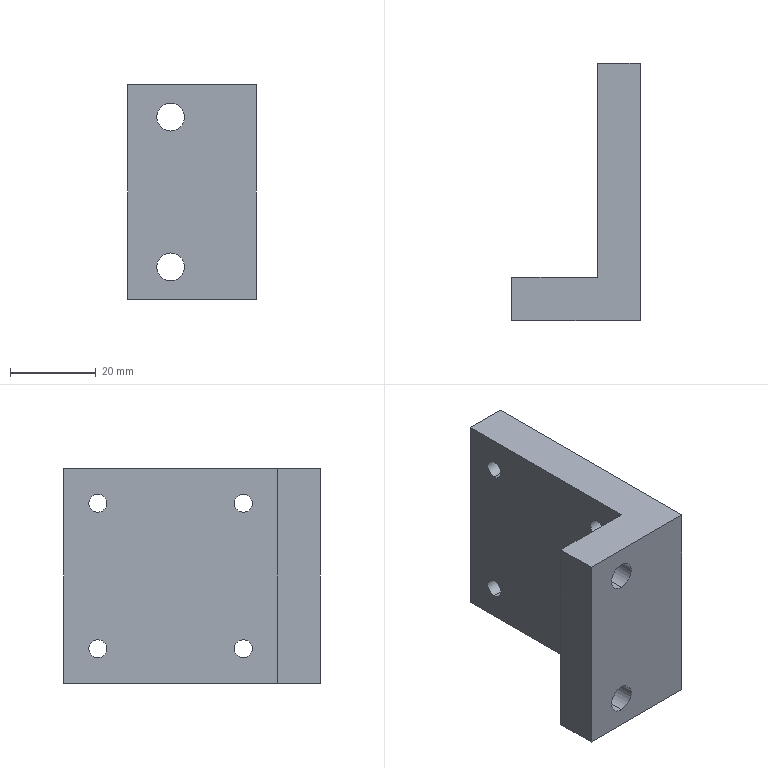Part | STEP file | BU-A20 | 1 solid | 20 faces | box 30 x 60 x 50 mm | volume 38782 mm3 | cylinder 12 | plane 8 | commonest cylinder face diameters 4.2 x8 6.5 x4